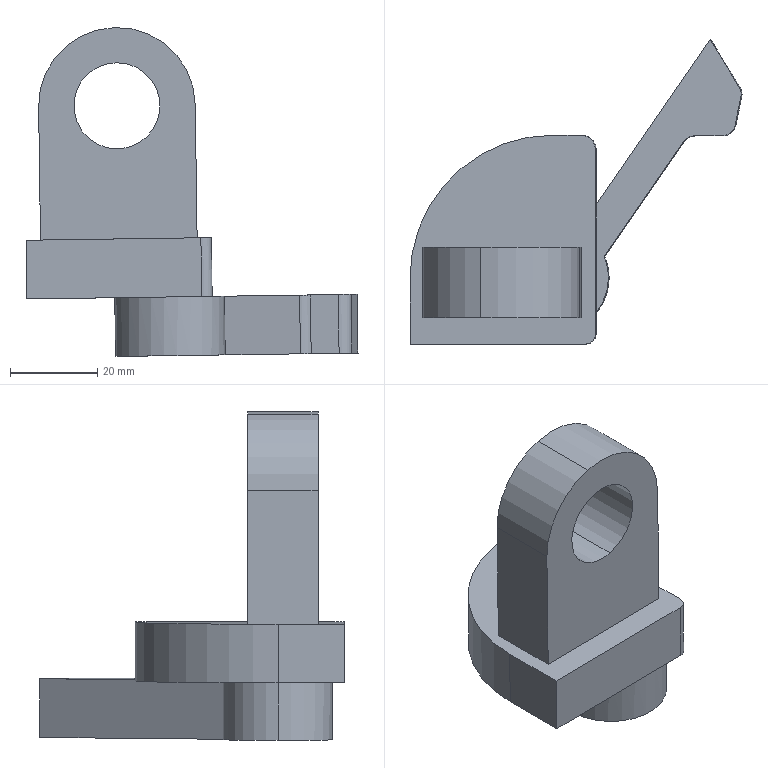Part | SolidWorks | features BaseBody 1 | 1 solid | 30 faces | box 76.312 x 69.944 x 75.61 mm | volume 59261 mm3 | plane 17 | cylinder 13 | commonest cylinder face diameters 6 x3 25.2 x3 19.8 x2 36 x2 4.8 x1 6.473 x1
STEP:
#1=CARTESIAN_POINT('',(-204.185,169.283,1047.886));
#2=VERTEX_POINT('',#1);
#3=CARTESIAN_POINT('',(-229.382,169.283,1047.53));
#4=VERTEX_POINT('',#3);
#5=CARTESIAN_POINT('',(-216.783,169.283,1047.708));
#6=DIRECTION('',(0.0141,0.,-0.9999));
#7=DIRECTION('',(0.9999,0.,0.0141));
#8=AXIS2_PLACEMENT_3D('',#5,#6,#7);
#9=CIRCLE('',#8,12.6);
#10=EDGE_CURVE('',#2,#4,#9,.T.);
#11=ORIENTED_EDGE('',*,*,#10,.F.);
#12=CARTESIAN_POINT('',(-204.375,169.283,1061.384));
#13=VERTEX_POINT('',#12);
#14=CARTESIAN_POINT('',(-204.185,169.283,1047.886));
#15=DIRECTION('',(-0.0141,0.,0.9999));
#16=VECTOR('',#15,1000.);
#17=LINE('',#14,#16);
#18=EDGE_CURVE('',#2,#13,#17,.T.);
#19=ORIENTED_EDGE('',*,*,#18,.T.);
#20=CARTESIAN_POINT('',(-207.186,161.349,1061.345));
#21=VERTEX_POINT('',#20);
#22=CARTESIAN_POINT('',(-216.974,169.283,1061.207));
#23=DIRECTION('',(0.0141,0.,-0.9999));
#24=DIRECTION('',(0.9999,0.,0.0141));
#25=AXIS2_PLACEMENT_3D('',#22,#23,#24);
#26=CIRCLE('',#25,12.6);
#27=EDGE_CURVE('',#13,#21,#26,.T.);
#28=ORIENTED_EDGE('',*,*,#27,.T.);
#29=CARTESIAN_POINT('',(-229.572,169.283,1061.029));
#30=VERTEX_POINT('',#29);
#31=CARTESIAN_POINT('',(-216.974,169.283,1061.207));
#32=DIRECTION('',(0.0141,0.,-0.9999));
#33=DIRECTION('',(0.9999,0.,0.0141));
#34=AXIS2_PLACEMENT_3D('',#31,#32,#33);
#35=CIRCLE('',#34,12.6);
#36=EDGE_CURVE('',#21,#30,#35,.T.);
#37=ORIENTED_EDGE('',*,*,#36,.T.);
#38=CARTESIAN_POINT('',(-229.382,169.283,1047.53));
#39=DIRECTION('',(-0.0141,0.,0.9999));
#40=VECTOR('',#39,1000.);
#41=LINE('',#38,#40);
#42=EDGE_CURVE('',#4,#30,#41,.T.);
#43=ORIENTED_EDGE('',*,*,#42,.F.);
#44=EDGE_LOOP('',(#11,#19,#28,#37,#43));
#45=FACE_OUTER_BOUND('',#44,.T.);
#46=CARTESIAN_POINT('',(-216.783,169.283,1047.708));
#47=DIRECTION('',(-0.0141,0.,0.9999));
#48=DIRECTION('',(-0.9999,0.,-0.0141));
#49=AXIS2_PLACEMENT_3D('',#46,#47,#48);
#50=CYLINDRICAL_SURFACE('',#49,12.6);
#51=ADVANCED_FACE('',(#45),#50,.T.);
#52=CARTESIAN_POINT('',(-210.908,180.429,1047.791));
#53=VERTEX_POINT('',#52);
#54=CARTESIAN_POINT('',(-216.783,169.283,1047.708));
#55=DIRECTION('',(0.0141,0.,-0.9999));
#56=DIRECTION('',(0.9999,0.,0.0141));
#57=AXIS2_PLACEMENT_3D('',#54,#55,#56);
#58=CIRCLE('',#57,12.6);
#59=EDGE_CURVE('',#4,#53,#58,.T.);
#60=ORIENTED_EDGE('',*,*,#59,.F.);
#61=ORIENTED_EDGE('',*,*,#42,.T.);
#62=CARTESIAN_POINT('',(-211.099,180.429,1061.289));
#63=VERTEX_POINT('',#62);
#64=CARTESIAN_POINT('',(-216.974,169.283,1061.207));
#65=DIRECTION('',(0.0141,0.,-0.9999));
#66=DIRECTION('',(0.9999,0.,0.0141));
#67=AXIS2_PLACEMENT_3D('',#64,#65,#66);
#68=CIRCLE('',#67,12.6);
#69=EDGE_CURVE('',#30,#63,#68,.T.);
#70=ORIENTED_EDGE('',*,*,#69,.T.);
#71=CARTESIAN_POINT('',(-210.908,180.429,1047.791));
#72=DIRECTION('',(-0.0141,0.,0.9999));
#73=VECTOR('',#72,1000.);
#74=LINE('',#71,#73);
#75=EDGE_CURVE('',#53,#63,#74,.T.);
#76=ORIENTED_EDGE('',*,*,#75,.F.);
#77=EDGE_LOOP('',(#60,#61,#70,#76));
#78=FACE_OUTER_BOUND('',#77,.T.);
#79=CARTESIAN_POINT('',(-216.783,169.283,1047.708));
#80=DIRECTION('',(-0.0141,0.,0.9999));
#81=DIRECTION('',(-0.9999,0.,-0.0141));
#82=AXIS2_PLACEMENT_3D('',#79,#80,#81);
#83=CYLINDRICAL_SURFACE('',#82,12.6);
#84=ADVANCED_FACE('',(#78),#83,.T.);
#85=CARTESIAN_POINT('',(-226.509,176.294,1095.578));
#86=VERTEX_POINT('',#85);
#87=CARTESIAN_POINT('',(-231.633,176.294,1114.703));
#88=VERTEX_POINT('',#87);
#89=CARTESIAN_POINT('',(-229.071,176.294,1105.14));
#90=DIRECTION('',(0.,-1.,0.));
#91=DIRECTION('',(0.9999,0.,0.0141));
#92=AXIS2_PLACEMENT_3D('',#89,#90,#91);
#93=CIRCLE('',#92,9.9);
#94=EDGE_CURVE('',#86,#88,#93,.T.);
#95=ORIENTED_EDGE('',*,*,#94,.F.);
#96=CARTESIAN_POINT('',(-226.509,160.094,1095.578));
#97=VERTEX_POINT('',#96);
#98=CARTESIAN_POINT('',(-226.509,176.294,1095.578));
#99=DIRECTION('',(0.,-1.,0.));
#100=VECTOR('',#99,1000.);
#101=LINE('',#98,#100);
#102=EDGE_CURVE('',#86,#97,#101,.T.);
#103=ORIENTED_EDGE('',*,*,#102,.T.);
#104=CARTESIAN_POINT('',(-231.633,160.094,1114.703));
#105=VERTEX_POINT('',#104);
#106=CARTESIAN_POINT('',(-229.071,160.094,1105.14));
#107=DIRECTION('',(0.,-1.,0.));
#108=DIRECTION('',(0.9999,0.,0.0141));
#109=AXIS2_PLACEMENT_3D('',#106,#107,#108);
#110=CIRCLE('',#109,9.9);
#111=EDGE_CURVE('',#97,#105,#110,.T.);
#112=ORIENTED_EDGE('',*,*,#111,.T.);
#113=CARTESIAN_POINT('',(-231.633,176.294,1114.703));
#114=DIRECTION('',(0.,-1.,0.));
#115=VECTOR('',#114,1000.);
#116=LINE('',#113,#115);
#117=EDGE_CURVE('',#88,#105,#116,.T.);
#118=ORIENTED_EDGE('',*,*,#117,.F.);
#119=EDGE_LOOP('',(#95,#103,#112,#118));
#120=FACE_OUTER_BOUND('',#119,.T.);
#121=CARTESIAN_POINT('',(-229.071,176.294,1105.14));
#122=DIRECTION('',(0.,-1.,0.));
#123=DIRECTION('',(-0.2588,0.,0.9659));
#124=AXIS2_PLACEMENT_3D('',#121,#122,#123);
#125=CYLINDRICAL_SURFACE('',#124,9.9);
#126=ADVANCED_FACE('',(#120),#125,.F.);
#127=CARTESIAN_POINT('',(-211.073,176.294,1105.394));
#128=VERTEX_POINT('',#127);
#129=CARTESIAN_POINT('',(-233.73,176.294,1122.527));
#130=VERTEX_POINT('',#129);
#131=CARTESIAN_POINT('',(-229.071,176.294,1105.14));
#132=DIRECTION('',(0.,-1.,0.));
#133=DIRECTION('',(0.9999,0.,0.0141));
#134=AXIS2_PLACEMENT_3D('',#131,#132,#133);
#135=CIRCLE('',#134,18.);
#136=EDGE_CURVE('',#128,#130,#135,.T.);
#137=ORIENTED_EDGE('',*,*,#136,.T.);
#138=CARTESIAN_POINT('',(-233.73,160.094,1122.527));
#139=VERTEX_POINT('',#138);
#140=CARTESIAN_POINT('',(-233.73,176.294,1122.527));
#141=DIRECTION('',(0.,-1.,0.));
#142=VECTOR('',#141,1000.);
#143=LINE('',#140,#142);
#144=EDGE_CURVE('',#130,#139,#143,.T.);
#145=ORIENTED_EDGE('',*,*,#144,.T.);
#146=CARTESIAN_POINT('',(-211.073,160.094,1105.394));
#147=VERTEX_POINT('',#146);
#148=CARTESIAN_POINT('',(-229.071,160.094,1105.14));
#149=DIRECTION('',(0.,-1.,0.));
#150=DIRECTION('',(0.9999,0.,0.0141));
#151=AXIS2_PLACEMENT_3D('',#148,#149,#150);
#152=CIRCLE('',#151,18.);
#153=EDGE_CURVE('',#147,#139,#152,.T.);
#154=ORIENTED_EDGE('',*,*,#153,.F.);
#155=CARTESIAN_POINT('',(-211.073,176.294,1105.394));
#156=DIRECTION('',(0.,-1.,0.));
#157=VECTOR('',#156,1000.);
#158=LINE('',#155,#157);
#159=EDGE_CURVE('',#128,#147,#158,.T.);
#160=ORIENTED_EDGE('',*,*,#159,.F.);
#161=EDGE_LOOP('',(#137,#145,#154,#160));
#162=FACE_OUTER_BOUND('',#161,.T.);
#163=CARTESIAN_POINT('',(-229.071,176.294,1105.14));
#164=DIRECTION('',(0.,-1.,0.));
#165=DIRECTION('',(-0.2588,0.,0.9659));
#166=AXIS2_PLACEMENT_3D('',#163,#164,#165);
#167=CYLINDRICAL_SURFACE('',#166,18.);
#168=ADVANCED_FACE('',(#162),#167,.T.);
#169=CARTESIAN_POINT('',(-175.066,204.386,1048.296));
#170=VERTEX_POINT('',#169);
#171=CARTESIAN_POINT('',(-178.006,201.983,1048.255));
#172=VERTEX_POINT('',#171);
#173=CARTESIAN_POINT('',(-178.006,204.983,1048.255));
#174=DIRECTION('',(0.0141,0.,-0.9999));
#175=DIRECTION('',(-0.9999,0.,-0.0141));
#176=AXIS2_PLACEMENT_3D('',#173,#174,#175);
#177=CIRCLE('',#176,3.);
#178=EDGE_CURVE('',#170,#172,#177,.T.);
#179=ORIENTED_EDGE('',*,*,#178,.F.);
#180=CARTESIAN_POINT('',(-175.257,204.386,1061.795));
#181=VERTEX_POINT('',#180);
#182=CARTESIAN_POINT('',(-175.066,204.386,1048.296));
#183=DIRECTION('',(0.0141,0.,-0.9999));
#184=VECTOR('',#183,1000.);
#185=LINE('',#182,#184);
#186=EDGE_CURVE('',#181,#170,#185,.T.);
#187=ORIENTED_EDGE('',*,*,#186,.F.);
#188=CARTESIAN_POINT('',(-178.196,201.983,1061.753));
#189=VERTEX_POINT('',#188);
#190=CARTESIAN_POINT('',(-178.196,204.983,1061.753));
#191=DIRECTION('',(-0.0141,0.,0.9999));
#192=DIRECTION('',(-0.9999,0.,-0.0141));
#193=AXIS2_PLACEMENT_3D('',#190,#191,#192);
#194=CIRCLE('',#193,3.);
#195=EDGE_CURVE('',#189,#181,#194,.T.);
#196=ORIENTED_EDGE('',*,*,#195,.F.);
#197=CARTESIAN_POINT('',(-178.006,201.983,1048.255));
#198=DIRECTION('',(-0.0141,0.,0.9999));
#199=VECTOR('',#198,1000.);
#200=LINE('',#197,#199);
#201=EDGE_CURVE('',#172,#189,#200,.T.);
#202=ORIENTED_EDGE('',*,*,#201,.F.);
#203=EDGE_LOOP('',(#179,#187,#196,#202));
#204=FACE_OUTER_BOUND('',#203,.T.);
#205=CARTESIAN_POINT('',(-178.006,204.983,1048.255));
#206=DIRECTION('',(-0.0141,0.,0.9999));
#207=DIRECTION('',(-0.9999,0.,-0.0141));
#208=AXIS2_PLACEMENT_3D('',#205,#206,#207);
#209=CYLINDRICAL_SURFACE('',#208,3.);
#210=ADVANCED_FACE('',(#204),#209,.T.);
#211=CARTESIAN_POINT('',(-184.425,201.983,1048.164));
#212=VERTEX_POINT('',#211);
#213=CARTESIAN_POINT('',(-186.893,200.688,1048.129));
#214=VERTEX_POINT('',#213);
#215=CARTESIAN_POINT('',(-184.425,198.983,1048.164));
#216=DIRECTION('',(-0.0141,0.,0.9999));
#217=DIRECTION('',(-0.9999,0.,-0.0141));
#218=AXIS2_PLACEMENT_3D('',#215,#216,#217);
#219=CIRCLE('',#218,3.);
#220=EDGE_CURVE('',#212,#214,#219,.T.);
#221=ORIENTED_EDGE('',*,*,#220,.F.);
#222=CARTESIAN_POINT('',(-184.615,201.983,1061.663));
#223=VERTEX_POINT('',#222);
#224=CARTESIAN_POINT('',(-184.425,201.983,1048.164));
#225=DIRECTION('',(0.0141,0.,-0.9999));
#226=VECTOR('',#225,1000.);
#227=LINE('',#224,#226);
#228=EDGE_CURVE('',#223,#212,#227,.T.);
#229=ORIENTED_EDGE('',*,*,#228,.F.);
#230=CARTESIAN_POINT('',(-187.083,200.688,1061.628));
#231=VERTEX_POINT('',#230);
#232=CARTESIAN_POINT('',(-184.615,198.983,1061.663));
#233=DIRECTION('',(0.0141,0.,-0.9999));
#234=DIRECTION('',(-0.9999,0.,-0.0141));
#235=AXIS2_PLACEMENT_3D('',#232,#233,#234);
#236=CIRCLE('',#235,3.);
#237=EDGE_CURVE('',#231,#223,#236,.T.);
#238=ORIENTED_EDGE('',*,*,#237,.F.);
#239=CARTESIAN_POINT('',(-187.083,200.688,1061.628));
#240=DIRECTION('',(-0.0141,0.,0.9999));
#241=VECTOR('',#240,1000.);
#242=LINE('',#239,#241);
#243=EDGE_CURVE('',#214,#231,#242,.T.);
#244=ORIENTED_EDGE('',*,*,#243,.F.);
#245=EDGE_LOOP('',(#221,#229,#238,#244));
#246=FACE_OUTER_BOUND('',#245,.T.);
#247=CARTESIAN_POINT('',(-184.425,198.983,1048.164));
#248=DIRECTION('',(0.0141,0.,-0.9999));
#249=DIRECTION('',(0.9999,0.,0.0141));
#250=AXIS2_PLACEMENT_3D('',#247,#248,#249);
#251=CYLINDRICAL_SURFACE('',#250,3.);
#252=ADVANCED_FACE('',(#246),#251,.F.);
#253=CARTESIAN_POINT('',(-174.106,213.185,1048.31));
#254=VERTEX_POINT('',#253);
#255=CARTESIAN_POINT('',(-173.72,211.014,1048.315));
#256=VERTEX_POINT('',#255);
#257=CARTESIAN_POINT('',(-176.659,211.611,1048.274));
#258=DIRECTION('',(0.0141,0.,-0.9999));
#259=DIRECTION('',(-0.9999,0.,-0.0141));
#260=AXIS2_PLACEMENT_3D('',#257,#258,#259);
#261=CIRCLE('',#260,3.);
#262=EDGE_CURVE('',#254,#256,#261,.T.);
#263=ORIENTED_EDGE('',*,*,#262,.F.);
#264=CARTESIAN_POINT('',(-174.296,213.185,1061.808));
#265=VERTEX_POINT('',#264);
#266=CARTESIAN_POINT('',(-174.106,213.185,1048.31));
#267=DIRECTION('',(0.0141,0.,-0.9999));
#268=VECTOR('',#267,1000.);
#269=LINE('',#266,#268);
#270=EDGE_CURVE('',#265,#254,#269,.T.);
#271=ORIENTED_EDGE('',*,*,#270,.F.);
#272=CARTESIAN_POINT('',(-173.91,211.014,1061.814));
#273=VERTEX_POINT('',#272);
#274=CARTESIAN_POINT('',(-176.85,211.611,1061.772));
#275=DIRECTION('',(-0.0141,0.,0.9999));
#276=DIRECTION('',(-0.9999,0.,-0.0141));
#277=AXIS2_PLACEMENT_3D('',#274,#275,#276);
#278=CIRCLE('',#277,3.);
#279=EDGE_CURVE('',#273,#265,#278,.T.);
#280=ORIENTED_EDGE('',*,*,#279,.F.);
#281=CARTESIAN_POINT('',(-173.72,211.014,1048.315));
#282=DIRECTION('',(-0.0141,0.,0.9999));
#283=VECTOR('',#282,1000.);
#284=LINE('',#281,#283);
#285=EDGE_CURVE('',#256,#273,#284,.T.);
#286=ORIENTED_EDGE('',*,*,#285,.F.);
#287=EDGE_LOOP('',(#263,#271,#280,#286));
#288=FACE_OUTER_BOUND('',#287,.T.);
#289=CARTESIAN_POINT('',(-176.659,211.611,1048.274));
#290=DIRECTION('',(-0.0141,0.,0.9999));
#291=DIRECTION('',(-0.9999,0.,-0.0141));
#292=AXIS2_PLACEMENT_3D('',#289,#290,#291);
#293=CYLINDRICAL_SURFACE('',#292,3.);
#294=ADVANCED_FACE('',(#288),#293,.T.);
#295=CARTESIAN_POINT('',(-180.792,224.039,1048.216));
#296=VERTEX_POINT('',#295);
#297=CARTESIAN_POINT('',(-178.025,219.547,1048.255));
#298=DIRECTION('',(0.5245,-0.8514,0.007398));
#299=VECTOR('',#298,1000.);
#300=LINE('',#297,#299);
#301=EDGE_CURVE('',#296,#254,#300,.T.);
#302=ORIENTED_EDGE('',*,*,#301,.T.);
#303=ORIENTED_EDGE('',*,*,#262,.T.);
#304=CARTESIAN_POINT('',(-174.428,207.529,1048.305));
#305=DIRECTION('',(-0.1991,-0.98,-0.002808));
#306=VECTOR('',#305,1000.);
#307=LINE('',#304,#306);
#308=EDGE_CURVE('',#256,#170,#307,.T.);
#309=ORIENTED_EDGE('',*,*,#308,.T.);
#310=ORIENTED_EDGE('',*,*,#178,.T.);
#311=CARTESIAN_POINT('',(-190.236,201.983,1048.082));
#312=DIRECTION('',(-0.9999,0.,-0.0141));
#313=VECTOR('',#312,1000.);
#314=LINE('',#311,#313);
#315=EDGE_CURVE('',#172,#212,#314,.T.);
#316=ORIENTED_EDGE('',*,*,#315,.T.);
#317=ORIENTED_EDGE('',*,*,#220,.T.);
#318=CARTESIAN_POINT('',(-205.184,174.201,1047.871));
#319=VERTEX_POINT('',#318);
#320=CARTESIAN_POINT('',(-194.286,189.983,1048.025));
#321=DIRECTION('',(-0.5682,-0.8228,-0.008015));
#322=VECTOR('',#321,1000.);
#323=LINE('',#320,#322);
#324=EDGE_CURVE('',#214,#319,#323,.T.);
#325=ORIENTED_EDGE('',*,*,#324,.T.);
#326=CARTESIAN_POINT('',(-216.783,169.283,1047.708));
#327=DIRECTION('',(0.0141,0.,-0.9999));
#328=DIRECTION('',(0.9999,0.,0.0141));
#329=AXIS2_PLACEMENT_3D('',#326,#327,#328);
#330=CIRCLE('',#329,12.6);
#331=EDGE_CURVE('',#319,#2,#330,.T.);
#332=ORIENTED_EDGE('',*,*,#331,.T.);
#333=ORIENTED_EDGE('',*,*,#10,.T.);
#334=ORIENTED_EDGE('',*,*,#59,.T.);
#335=CARTESIAN_POINT('',(-210.908,180.429,1047.791));
#336=DIRECTION('',(0.5682,0.8228,0.008015));
#337=VECTOR('',#336,1000.);
#338=LINE('',#335,#337);
#339=EDGE_CURVE('',#53,#296,#338,.T.);
#340=ORIENTED_EDGE('',*,*,#339,.T.);
#341=EDGE_LOOP('',(#302,#303,#309,#310,#316,#317,#325,#332,#333,#334,#340));
#342=FACE_OUTER_BOUND('',#341,.T.);
#343=CARTESIAN_POINT('',(-216.783,169.283,1047.708));
#344=DIRECTION('',(0.0141,0.,-0.9999));
#345=DIRECTION('',(0.,-1.,0.));
#346=AXIS2_PLACEMENT_3D('',#343,#344,#345);
#347=PLANE('',#346);
#348=ADVANCED_FACE('',(#342),#347,.T.);
#349=CARTESIAN_POINT('',(-174.618,207.529,1061.804));
#350=DIRECTION('',(-0.1991,-0.98,-0.002808));
#351=VECTOR('',#350,1000.);
#352=LINE('',#349,#351);
#353=EDGE_CURVE('',#273,#181,#352,.T.);
#354=ORIENTED_EDGE('',*,*,#353,.F.);
#355=ORIENTED_EDGE('',*,*,#279,.T.);
#356=CARTESIAN_POINT('',(-180.983,224.039,1061.714));
#357=VERTEX_POINT('',#356);
#358=CARTESIAN_POINT('',(-178.216,219.547,1061.753));
#359=DIRECTION('',(0.5245,-0.8514,0.007398));
#360=VECTOR('',#359,1000.);
#361=LINE('',#358,#360);
#362=EDGE_CURVE('',#357,#265,#361,.T.);
#363=ORIENTED_EDGE('',*,*,#362,.F.);
#364=CARTESIAN_POINT('',(-207.186,186.095,1061.345));
#365=VERTEX_POINT('',#364);
#366=CARTESIAN_POINT('',(-211.099,180.429,1061.289));
#367=DIRECTION('',(0.5682,0.8228,0.008015));
#368=VECTOR('',#367,1000.);
#369=LINE('',#366,#368);
#370=EDGE_CURVE('',#365,#357,#369,.T.);
#371=ORIENTED_EDGE('',*,*,#370,.F.);
#372=CARTESIAN_POINT('',(-207.186,152.929,1061.345));
#373=DIRECTION('',(0.,1.,0.));
#374=VECTOR('',#373,1000.);
#375=LINE('',#372,#374);
#376=EDGE_CURVE('',#21,#365,#375,.T.);
#377=ORIENTED_EDGE('',*,*,#376,.F.);
#378=ORIENTED_EDGE('',*,*,#27,.F.);
#379=CARTESIAN_POINT('',(-205.375,174.201,1061.37));
#380=VERTEX_POINT('',#379);
#381=CARTESIAN_POINT('',(-216.974,169.283,1061.207));
#382=DIRECTION('',(0.0141,0.,-0.9999));
#383=DIRECTION('',(0.9999,0.,0.0141));
#384=AXIS2_PLACEMENT_3D('',#381,#382,#383);
#385=CIRCLE('',#384,12.6);
#386=EDGE_CURVE('',#380,#13,#385,.T.);
#387=ORIENTED_EDGE('',*,*,#386,.F.);
#388=CARTESIAN_POINT('',(-194.476,189.983,1061.524));
#389=DIRECTION('',(-0.5682,-0.8228,-0.008015));
#390=VECTOR('',#389,1000.);
#391=LINE('',#388,#390);
#392=EDGE_CURVE('',#231,#380,#391,.T.);
#393=ORIENTED_EDGE('',*,*,#392,.F.);
#394=ORIENTED_EDGE('',*,*,#237,.T.);
#395=CARTESIAN_POINT('',(-190.426,201.983,1061.581));
#396=DIRECTION('',(-0.9999,0.,-0.0141));
#397=VECTOR('',#396,1000.);
#398=LINE('',#395,#397);
#399=EDGE_CURVE('',#189,#223,#398,.T.);
#400=ORIENTED_EDGE('',*,*,#399,.F.);
#401=ORIENTED_EDGE('',*,*,#195,.T.);
#402=EDGE_LOOP('',(#354,#355,#363,#371,#377,#378,#387,#393,#394,#400,#401));
#403=FACE_OUTER_BOUND('',#402,.T.);
#404=CARTESIAN_POINT('',(-216.974,169.283,1061.207));
#405=DIRECTION('',(0.0141,0.,-0.9999));
#406=DIRECTION('',(0.,-1.,0.));
#407=AXIS2_PLACEMENT_3D('',#404,#405,#406);
#408=PLANE('',#407);
#409=ADVANCED_FACE('',(#403),#408,.F.);
#410=ORIENTED_EDGE('',*,*,#324,.F.);
#411=ORIENTED_EDGE('',*,*,#243,.T.);
#412=ORIENTED_EDGE('',*,*,#392,.T.);
#413=CARTESIAN_POINT('',(-205.184,174.201,1047.871));
#414=DIRECTION('',(-0.0141,0.,0.9999));
#415=VECTOR('',#414,1000.);
#416=LINE('',#413,#415);
#417=EDGE_CURVE('',#319,#380,#416,.T.);
#418=ORIENTED_EDGE('',*,*,#417,.F.);
#419=EDGE_LOOP('',(#410,#411,#412,#418));
#420=FACE_OUTER_BOUND('',#419,.T.);
#421=CARTESIAN_POINT('',(-194.286,189.983,1048.025));
#422=DIRECTION('',(-0.8227,0.5683,-0.0116));
#423=DIRECTION('',(-0.0141,0.,0.9999));
#424=AXIS2_PLACEMENT_3D('',#421,#422,#423);
#425=PLANE('',#424);
#426=ADVANCED_FACE('',(#420),#425,.F.);
#427=ORIENTED_EDGE('',*,*,#399,.T.);
#428=ORIENTED_EDGE('',*,*,#228,.T.);
#429=ORIENTED_EDGE('',*,*,#315,.F.);
#430=ORIENTED_EDGE('',*,*,#201,.T.);
#431=EDGE_LOOP('',(#427,#428,#429,#430));
#432=FACE_OUTER_BOUND('',#431,.T.);
#433=CARTESIAN_POINT('',(-190.236,201.983,1048.082));
#434=DIRECTION('',(0.,1.,0.));
#435=DIRECTION('',(1.,0.,0.));
#436=AXIS2_PLACEMENT_3D('',#433,#434,#435);
#437=PLANE('',#436);
#438=ADVANCED_FACE('',(#432),#437,.F.);
#439=ORIENTED_EDGE('',*,*,#308,.F.);
#440=ORIENTED_EDGE('',*,*,#285,.T.);
#441=ORIENTED_EDGE('',*,*,#353,.T.);
#442=ORIENTED_EDGE('',*,*,#186,.T.);
#443=EDGE_LOOP('',(#439,#440,#441,#442));
#444=FACE_OUTER_BOUND('',#443,.T.);
#445=CARTESIAN_POINT('',(-174.428,207.529,1048.305));
#446=DIRECTION('',(-0.9799,0.1991,-0.01382));
#447=DIRECTION('',(-0.0141,0.,0.9999));
#448=AXIS2_PLACEMENT_3D('',#445,#446,#447);
#449=PLANE('',#448);
#450=ADVANCED_FACE('',(#444),#449,.F.);
#451=ORIENTED_EDGE('',*,*,#362,.T.);
#452=ORIENTED_EDGE('',*,*,#270,.T.);
#453=ORIENTED_EDGE('',*,*,#301,.F.);
#454=CARTESIAN_POINT('',(-180.792,224.039,1048.216));
#455=DIRECTION('',(-0.0141,0.,0.9999));
#456=VECTOR('',#455,1000.);
#457=LINE('',#454,#456);
#458=EDGE_CURVE('',#296,#357,#457,.T.);
#459=ORIENTED_EDGE('',*,*,#458,.T.);
#460=EDGE_LOOP('',(#451,#452,#453,#459));
#461=FACE_OUTER_BOUND('',#460,.T.);
#462=CARTESIAN_POINT('',(-178.025,219.547,1048.255));
#463=DIRECTION('',(-0.8513,-0.5246,-0.01201));
#464=DIRECTION('',(-0.5246,0.8513,0.));
#465=AXIS2_PLACEMENT_3D('',#462,#463,#464);
#466=PLANE('',#465);
#467=ADVANCED_FACE('',(#461),#466,.F.);
#468=CARTESIAN_POINT('',(-211.099,180.429,1061.289));
#469=DIRECTION('',(0.5682,0.8228,0.008015));
#470=VECTOR('',#469,1000.);
#471=LINE('',#468,#470);
#472=EDGE_CURVE('',#63,#365,#471,.T.);
#473=ORIENTED_EDGE('',*,*,#472,.T.);
#474=ORIENTED_EDGE('',*,*,#370,.T.);
#475=ORIENTED_EDGE('',*,*,#458,.F.);
#476=ORIENTED_EDGE('',*,*,#339,.F.);
#477=ORIENTED_EDGE('',*,*,#75,.T.);
#478=EDGE_LOOP('',(#473,#474,#475,#476,#477));
#479=FACE_OUTER_BOUND('',#478,.T.);
#480=CARTESIAN_POINT('',(-210.908,180.429,1047.791));
#481=DIRECTION('',(0.8227,-0.5683,0.0116));
#482=DIRECTION('',(0.,-0.02042,-0.9998));
#483=AXIS2_PLACEMENT_3D('',#480,#481,#482);
#484=PLANE('',#483);
#485=ADVANCED_FACE('',(#479),#484,.F.);
#486=CARTESIAN_POINT('',(-207.186,156.494,1061.345));
#487=VERTEX_POINT('',#486);
#488=CARTESIAN_POINT('',(-209.586,154.094,1061.311));
#489=VERTEX_POINT('',#488);
#490=CARTESIAN_POINT('',(-209.586,156.494,1061.311));
#491=DIRECTION('',(0.0141,0.,-0.9999));
#492=DIRECTION('',(0.9999,0.,0.0141));
#493=AXIS2_PLACEMENT_3D('',#490,#491,#492);
#494=CIRCLE('',#493,2.4);
#495=EDGE_CURVE('',#487,#489,#494,.T.);
#496=ORIENTED_EDGE('',*,*,#495,.F.);
#497=CARTESIAN_POINT('',(-207.376,156.494,1074.843));
#498=VERTEX_POINT('',#497);
#499=CARTESIAN_POINT('',(-207.186,156.494,1061.345));
#500=DIRECTION('',(0.0141,0.,-0.9999));
#501=VECTOR('',#500,1000.);
#502=LINE('',#499,#501);
#503=EDGE_CURVE('',#498,#487,#502,.T.);
#504=ORIENTED_EDGE('',*,*,#503,.F.);
#505=CARTESIAN_POINT('',(-209.776,154.094,1074.809));
#506=VERTEX_POINT('',#505);
#507=CARTESIAN_POINT('',(-209.776,156.494,1074.809));
#508=DIRECTION('',(-0.0141,0.,0.9999));
#509=DIRECTION('',(0.9999,0.,0.0141));
#510=AXIS2_PLACEMENT_3D('',#507,#508,#509);
#511=CIRCLE('',#510,2.4);
#512=EDGE_CURVE('',#506,#498,#511,.T.);
#513=ORIENTED_EDGE('',*,*,#512,.F.);
#514=CARTESIAN_POINT('',(-209.586,154.094,1061.311));
#515=DIRECTION('',(-0.0141,0.,0.9999));
#516=VECTOR('',#515,1000.);
#517=LINE('',#514,#516);
#518=EDGE_CURVE('',#489,#506,#517,.T.);
#519=ORIENTED_EDGE('',*,*,#518,.F.);
#520=EDGE_LOOP('',(#496,#504,#513,#519));
#521=FACE_OUTER_BOUND('',#520,.T.);
#522=CARTESIAN_POINT('',(-209.586,156.494,1061.311));
#523=DIRECTION('',(-0.0141,0.,0.9999));
#524=DIRECTION('',(-0.9999,0.,-0.0141));
#525=AXIS2_PLACEMENT_3D('',#522,#523,#524);
#526=CYLINDRICAL_SURFACE('',#525,2.4);
#527=ADVANCED_FACE('',(#521),#526,.T.);
#528=CARTESIAN_POINT('',(-229.071,160.094,1105.14));
#529=DIRECTION('',(0.,-1.,0.));
#530=DIRECTION('',(0.9999,0.,0.0141));
#531=AXIS2_PLACEMENT_3D('',#528,#529,#530);
#532=CIRCLE('',#531,9.9);
#533=EDGE_CURVE('',#105,#97,#532,.T.);
#534=ORIENTED_EDGE('',*,*,#533,.F.);
#535=ORIENTED_EDGE('',*,*,#111,.F.);
#536=EDGE_LOOP('',(#534,#535));
#537=FACE_BOUND('',#536,.T.);
#538=CARTESIAN_POINT('',(-247.069,160.094,1104.886));
#539=VERTEX_POINT('',#538);
#540=CARTESIAN_POINT('',(-246.638,160.094,1074.289));
#541=VERTEX_POINT('',#540);
#542=CARTESIAN_POINT('',(-247.069,160.094,1104.886));
#543=DIRECTION('',(0.0141,0.,-0.9999));
#544=VECTOR('',#543,1000.);
#545=LINE('',#542,#544);
#546=EDGE_CURVE('',#539,#541,#545,.T.);
#547=ORIENTED_EDGE('',*,*,#546,.T.);
#548=CARTESIAN_POINT('',(-210.641,160.094,1074.797));
#549=VERTEX_POINT('',#548);
#550=CARTESIAN_POINT('',(-251.137,160.094,1074.226));
#551=DIRECTION('',(0.9999,0.,0.0141));
#552=VECTOR('',#551,1000.);
#553=LINE('',#550,#552);
#554=EDGE_CURVE('',#541,#549,#553,.T.);
#555=ORIENTED_EDGE('',*,*,#554,.T.);
#556=CARTESIAN_POINT('',(-210.573,160.094,1069.937));
#557=DIRECTION('',(-0.0141,0.,0.9999));
#558=VECTOR('',#557,1000.);
#559=LINE('',#556,#558);
#560=EDGE_CURVE('',#549,#147,#559,.T.);
#561=ORIENTED_EDGE('',*,*,#560,.T.);
#562=ORIENTED_EDGE('',*,*,#153,.T.);
#563=CARTESIAN_POINT('',(-229.071,160.094,1105.14));
#564=DIRECTION('',(0.,-1.,0.));
#565=DIRECTION('',(0.9999,0.,0.0141));
#566=AXIS2_PLACEMENT_3D('',#563,#564,#565);
#567=CIRCLE('',#566,18.);
#568=EDGE_CURVE('',#139,#539,#567,.T.);
#569=ORIENTED_EDGE('',*,*,#568,.T.);
#570=EDGE_LOOP('',(#547,#555,#561,#562,#569));
#571=FACE_OUTER_BOUND('',#570,.T.);
#572=CARTESIAN_POINT('',(-229.071,160.094,1105.14));
#573=DIRECTION('',(0.,-1.,0.));
#574=DIRECTION('',(0.,0.,-1.));
#575=AXIS2_PLACEMENT_3D('',#572,#573,#574);
#576=PLANE('',#575);
#577=ADVANCED_FACE('',(#537,#571),#576,.T.);
#578=CARTESIAN_POINT('',(-229.071,176.294,1105.14));
#579=DIRECTION('',(0.,-1.,0.));
#580=DIRECTION('',(0.9999,0.,0.0141));
#581=AXIS2_PLACEMENT_3D('',#578,#579,#580);
#582=CIRCLE('',#581,9.9);
#583=EDGE_CURVE('',#88,#86,#582,.T.);
#584=ORIENTED_EDGE('',*,*,#583,.T.);
#585=ORIENTED_EDGE('',*,*,#94,.T.);
#586=EDGE_LOOP('',(#584,#585));
#587=FACE_BOUND('',#586,.T.);
#588=CARTESIAN_POINT('',(-246.638,176.294,1074.289));
#589=VERTEX_POINT('',#588);
#590=CARTESIAN_POINT('',(-210.641,176.294,1074.797));
#591=VERTEX_POINT('',#590);
#592=CARTESIAN_POINT('',(-251.137,176.294,1074.226));
#593=DIRECTION('',(0.9999,0.,0.0141));
#594=VECTOR('',#593,1000.);
#595=LINE('',#592,#594);
#596=EDGE_CURVE('',#589,#591,#595,.T.);
#597=ORIENTED_EDGE('',*,*,#596,.F.);
#598=CARTESIAN_POINT('',(-247.069,176.294,1104.886));
#599=VERTEX_POINT('',#598);
#600=CARTESIAN_POINT('',(-247.069,176.294,1104.886));
#601=DIRECTION('',(0.0141,0.,-0.9999));
#602=VECTOR('',#601,1000.);
#603=LINE('',#600,#602);
#604=EDGE_CURVE('',#599,#589,#603,.T.);
#605=ORIENTED_EDGE('',*,*,#604,.F.);
#606=CARTESIAN_POINT('',(-229.071,176.294,1105.14));
#607=DIRECTION('',(0.,-1.,0.));
#608=DIRECTION('',(0.9999,0.,0.0141));
#609=AXIS2_PLACEMENT_3D('',#606,#607,#608);
#610=CIRCLE('',#609,18.);
#611=EDGE_CURVE('',#130,#599,#610,.T.);
#612=ORIENTED_EDGE('',*,*,#611,.F.);
#613=ORIENTED_EDGE('',*,*,#136,.F.);
#614=CARTESIAN_POINT('',(-210.573,176.294,1069.937));
#615=DIRECTION('',(-0.0141,0.,0.9999));
#616=VECTOR('',#615,1000.);
#617=LINE('',#614,#616);
#618=EDGE_CURVE('',#591,#128,#617,.T.);
#619=ORIENTED_EDGE('',*,*,#618,.F.);
#620=EDGE_LOOP('',(#597,#605,#612,#613,#619));
#621=FACE_OUTER_BOUND('',#620,.T.);
#622=CARTESIAN_POINT('',(-229.071,176.294,1105.14));
#623=DIRECTION('',(0.,-1.,0.));
#624=DIRECTION('',(0.,0.,-1.));
#625=AXIS2_PLACEMENT_3D('',#622,#623,#624);
#626=PLANE('',#625);
#627=ADVANCED_FACE('',(#587,#621),#626,.F.);
#628=ORIENTED_EDGE('',*,*,#560,.F.);
#629=CARTESIAN_POINT('',(-210.641,152.929,1074.797));
#630=DIRECTION('',(0.,1.,0.));
#631=VECTOR('',#630,1000.);
#632=LINE('',#629,#631);
#633=EDGE_CURVE('',#549,#591,#632,.T.);
#634=ORIENTED_EDGE('',*,*,#633,.T.);
#635=ORIENTED_EDGE('',*,*,#618,.T.);
#636=ORIENTED_EDGE('',*,*,#159,.T.);
#637=EDGE_LOOP('',(#628,#634,#635,#636));
#638=FACE_OUTER_BOUND('',#637,.T.);
#639=CARTESIAN_POINT('',(-210.573,176.294,1069.937));
#640=DIRECTION('',(0.9999,0.,0.0141));
#641=DIRECTION('',(0.,-1.,0.));
#642=AXIS2_PLACEMENT_3D('',#639,#640,#641);
#643=PLANE('',#642);
#644=ADVANCED_FACE('',(#638),#643,.T.);
#645=ORIENTED_EDGE('',*,*,#604,.T.);
#646=CARTESIAN_POINT('',(-246.638,152.929,1074.289));
#647=DIRECTION('',(0.,-1.,0.));
#648=VECTOR('',#647,1000.);
#649=LINE('',#646,#648);
#650=EDGE_CURVE('',#589,#541,#649,.T.);
#651=ORIENTED_EDGE('',*,*,#650,.T.);
#652=ORIENTED_EDGE('',*,*,#546,.F.);
#653=CARTESIAN_POINT('',(-247.069,176.294,1104.886));
#654=DIRECTION('',(0.,-1.,0.));
#655=VECTOR('',#654,1000.);
#656=LINE('',#653,#655);
#657=EDGE_CURVE('',#599,#539,#656,.T.);
#658=ORIENTED_EDGE('',*,*,#657,.F.);
#659=EDGE_LOOP('',(#645,#651,#652,#658));
#660=FACE_OUTER_BOUND('',#659,.T.);
#661=CARTESIAN_POINT('',(-247.069,176.294,1104.886));
#662=DIRECTION('',(-0.9999,0.,-0.0141));
#663=DIRECTION('',(-0.0141,0.,0.9999));
#664=AXIS2_PLACEMENT_3D('',#661,#662,#663);
#665=PLANE('',#664);
#666=ADVANCED_FACE('',(#660),#665,.T.);
#667=ORIENTED_EDGE('',*,*,#36,.F.);
#668=CARTESIAN_POINT('',(-207.186,152.929,1061.345));
#669=DIRECTION('',(0.,1.,0.));
#670=VECTOR('',#669,1000.);
#671=LINE('',#668,#670);
#672=EDGE_CURVE('',#487,#21,#671,.T.);
#673=ORIENTED_EDGE('',*,*,#672,.F.);
#674=ORIENTED_EDGE('',*,*,#495,.T.);
#675=CARTESIAN_POINT('',(-249.782,154.094,1060.744));
#676=VERTEX_POINT('',#675);
#677=CARTESIAN_POINT('',(-250.947,154.094,1060.727));
#678=DIRECTION('',(0.9999,0.,0.0141));
#679=VECTOR('',#678,1000.);
#680=LINE('',#677,#679);
#681=EDGE_CURVE('',#676,#489,#680,.T.);
#682=ORIENTED_EDGE('',*,*,#681,.F.);
#683=CARTESIAN_POINT('',(-249.782,169.283,1060.744));
#684=VERTEX_POINT('',#683);
#685=CARTESIAN_POINT('',(-249.782,152.929,1060.744));
#686=DIRECTION('',(0.,-1.,0.));
#687=VECTOR('',#686,1000.);
#688=LINE('',#685,#687);
#689=EDGE_CURVE('',#684,#676,#688,.T.);
#690=ORIENTED_EDGE('',*,*,#689,.F.);
#691=CARTESIAN_POINT('',(-216.974,202.094,1061.207));
#692=VERTEX_POINT('',#691);
#693=CARTESIAN_POINT('',(-216.974,169.283,1061.207));
#694=DIRECTION('',(-0.0141,0.,0.9999));
#695=DIRECTION('',(0.9999,0.,0.0141));
#696=AXIS2_PLACEMENT_3D('',#693,#694,#695);
#697=CIRCLE('',#696,32.811);
#698=EDGE_CURVE('',#692,#684,#697,.T.);
#699=ORIENTED_EDGE('',*,*,#698,.F.);
#700=CARTESIAN_POINT('',(-210.422,202.094,1061.299));
#701=VERTEX_POINT('',#700);
#702=CARTESIAN_POINT('',(-250.947,202.094,1060.727));
#703=DIRECTION('',(-0.9999,0.,-0.0141));
#704=VECTOR('',#703,1000.);
#705=LINE('',#702,#704);
#706=EDGE_CURVE('',#701,#692,#705,.T.);
#707=ORIENTED_EDGE('',*,*,#706,.F.);
#708=CARTESIAN_POINT('',(-207.186,198.858,1061.345));
#709=VERTEX_POINT('',#708);
#710=CARTESIAN_POINT('',(-210.422,198.858,1061.299));
#711=DIRECTION('',(-0.0141,0.,0.9999));
#712=DIRECTION('',(0.9999,0.,0.0141));
#713=AXIS2_PLACEMENT_3D('',#710,#711,#712);
#714=CIRCLE('',#713,3.236);
#715=EDGE_CURVE('',#709,#701,#714,.T.);
#716=ORIENTED_EDGE('',*,*,#715,.F.);
#717=CARTESIAN_POINT('',(-207.186,152.929,1061.345));
#718=DIRECTION('',(0.,1.,0.));
#719=VECTOR('',#718,1000.);
#720=LINE('',#717,#719);
#721=EDGE_CURVE('',#365,#709,#720,.T.);
#722=ORIENTED_EDGE('',*,*,#721,.F.);
#723=ORIENTED_EDGE('',*,*,#472,.F.);
#724=ORIENTED_EDGE('',*,*,#69,.F.);
#725=EDGE_LOOP('',(#667,#673,#674,#682,#690,#699,#707,#716,#722,#723,#724));
#726=FACE_OUTER_BOUND('',#725,.T.);
#727=CARTESIAN_POINT('',(-250.947,152.929,1060.727));
#728=DIRECTION('',(-0.0141,0.,0.9999));
#729=DIRECTION('',(0.,1.,0.));
#730=AXIS2_PLACEMENT_3D('',#727,#728,#729);
#731=PLANE('',#730);
#732=ADVANCED_FACE('',(#726),#731,.F.);
#733=CARTESIAN_POINT('',(-217.164,202.094,1074.705));
#734=VERTEX_POINT('',#733);
#735=CARTESIAN_POINT('',(-249.972,169.283,1074.242));
#736=VERTEX_POINT('',#735);
#737=CARTESIAN_POINT('',(-217.164,169.283,1074.705));
#738=DIRECTION('',(-0.0141,0.,0.9999));
#739=DIRECTION('',(0.9999,0.,0.0141));
#740=AXIS2_PLACEMENT_3D('',#737,#738,#739);
#741=CIRCLE('',#740,32.811);
#742=EDGE_CURVE('',#734,#736,#741,.T.);
#743=ORIENTED_EDGE('',*,*,#742,.F.);
#744=CARTESIAN_POINT('',(-216.974,202.094,1061.207));
#745=DIRECTION('',(-0.0141,0.,0.9999));
#746=VECTOR('',#745,1000.);
#747=LINE('',#744,#746);
#748=EDGE_CURVE('',#692,#734,#747,.T.);
#749=ORIENTED_EDGE('',*,*,#748,.F.);
#750=ORIENTED_EDGE('',*,*,#698,.T.);
#751=CARTESIAN_POINT('',(-249.782,169.283,1060.744));
#752=DIRECTION('',(-0.0141,0.,0.9999));
#753=VECTOR('',#752,1000.);
#754=LINE('',#751,#753);
#755=EDGE_CURVE('',#684,#736,#754,.T.);
#756=ORIENTED_EDGE('',*,*,#755,.T.);
#757=EDGE_LOOP('',(#743,#749,#750,#756));
#758=FACE_OUTER_BOUND('',#757,.T.);
#759=CARTESIAN_POINT('',(-216.974,169.283,1061.207));
#760=DIRECTION('',(-0.0141,0.,0.9999));
#761=DIRECTION('',(-0.9999,0.,-0.0141));
#762=AXIS2_PLACEMENT_3D('',#759,#760,#761);
#763=CYLINDRICAL_SURFACE('',#762,32.811);
#764=ADVANCED_FACE('',(#758),#763,.T.);
#765=CARTESIAN_POINT('',(-210.612,202.094,1074.798));
#766=VERTEX_POINT('',#765);
#767=CARTESIAN_POINT('',(-251.137,202.094,1074.226));
#768=DIRECTION('',(-0.9999,0.,-0.0141));
#769=VECTOR('',#768,1000.);
#770=LINE('',#767,#769);
#771=EDGE_CURVE('',#766,#734,#770,.T.);
#772=ORIENTED_EDGE('',*,*,#771,.F.);
#773=CARTESIAN_POINT('',(-210.422,202.094,1061.299));
#774=DIRECTION('',(-0.0141,0.,0.9999));
#775=VECTOR('',#774,1000.);
#776=LINE('',#773,#775);
#777=EDGE_CURVE('',#701,#766,#776,.T.);
#778=ORIENTED_EDGE('',*,*,#777,.F.);
#779=ORIENTED_EDGE('',*,*,#706,.T.);
#780=ORIENTED_EDGE('',*,*,#748,.T.);
#781=EDGE_LOOP('',(#772,#778,#779,#780));
#782=FACE_OUTER_BOUND('',#781,.T.);
#783=CARTESIAN_POINT('',(-210.422,202.094,1061.299));
#784=DIRECTION('',(0.,1.,0.));
#785=DIRECTION('',(1.,0.,0.));
#786=AXIS2_PLACEMENT_3D('',#783,#784,#785);
#787=PLANE('',#786);
#788=ADVANCED_FACE('',(#782),#787,.T.);
#789=CARTESIAN_POINT('',(-207.376,198.858,1074.843));
#790=VERTEX_POINT('',#789);
#791=CARTESIAN_POINT('',(-210.612,198.858,1074.798));
#792=DIRECTION('',(-0.0141,0.,0.9999));
#793=DIRECTION('',(0.9999,0.,0.0141));
#794=AXIS2_PLACEMENT_3D('',#791,#792,#793);
#795=CIRCLE('',#794,3.236);
#796=EDGE_CURVE('',#790,#766,#795,.T.);
#797=ORIENTED_EDGE('',*,*,#796,.F.);
#798=CARTESIAN_POINT('',(-207.186,198.858,1061.345));
#799=DIRECTION('',(-0.0141,0.,0.9999));
#800=VECTOR('',#799,1000.);
#801=LINE('',#798,#800);
#802=EDGE_CURVE('',#709,#790,#801,.T.);
#803=ORIENTED_EDGE('',*,*,#802,.F.);
#804=ORIENTED_EDGE('',*,*,#715,.T.);
#805=ORIENTED_EDGE('',*,*,#777,.T.);
#806=EDGE_LOOP('',(#797,#803,#804,#805));
#807=FACE_OUTER_BOUND('',#806,.T.);
#808=CARTESIAN_POINT('',(-210.422,198.858,1061.299));
#809=DIRECTION('',(-0.0141,0.,0.9999));
#810=DIRECTION('',(-0.9999,0.,-0.0141));
#811=AXIS2_PLACEMENT_3D('',#808,#809,#810);
#812=CYLINDRICAL_SURFACE('',#811,3.236);
#813=ADVANCED_FACE('',(#807),#812,.T.);
#814=CARTESIAN_POINT('',(-207.376,152.929,1074.843));
#815=DIRECTION('',(0.,1.,0.));
#816=VECTOR('',#815,1000.);
#817=LINE('',#814,#816);
#818=EDGE_CURVE('',#498,#790,#817,.T.);
#819=ORIENTED_EDGE('',*,*,#818,.F.);
#820=ORIENTED_EDGE('',*,*,#503,.T.);
#821=ORIENTED_EDGE('',*,*,#672,.T.);
#822=ORIENTED_EDGE('',*,*,#376,.T.);
#823=ORIENTED_EDGE('',*,*,#721,.T.);
#824=ORIENTED_EDGE('',*,*,#802,.T.);
#825=EDGE_LOOP('',(#819,#820,#821,#822,#823,#824));
#826=FACE_OUTER_BOUND('',#825,.T.);
#827=CARTESIAN_POINT('',(-207.186,146.594,1061.345));
#828=DIRECTION('',(0.9999,0.,0.0141));
#829=DIRECTION('',(0.,-1.,0.));
#830=AXIS2_PLACEMENT_3D('',#827,#828,#829);
#831=PLANE('',#830);
#832=ADVANCED_FACE('',(#826),#831,.T.);
#833=ORIENTED_EDGE('',*,*,#681,.T.);
#834=ORIENTED_EDGE('',*,*,#518,.T.);
#835=CARTESIAN_POINT('',(-249.972,154.094,1074.242));
#836=VERTEX_POINT('',#835);
#837=CARTESIAN_POINT('',(-251.137,154.094,1074.226));
#838=DIRECTION('',(0.9999,0.,0.0141));
#839=VECTOR('',#838,1000.);
#840=LINE('',#837,#839);
#841=EDGE_CURVE('',#836,#506,#840,.T.);
#842=ORIENTED_EDGE('',*,*,#841,.F.);
#843=CARTESIAN_POINT('',(-249.782,154.094,1060.744));
#844=DIRECTION('',(-0.0141,0.,0.9999));
#845=VECTOR('',#844,1000.);
#846=LINE('',#843,#845);
#847=EDGE_CURVE('',#676,#836,#846,.T.);
#848=ORIENTED_EDGE('',*,*,#847,.F.);
#849=EDGE_LOOP('',(#833,#834,#842,#848));
#850=FACE_OUTER_BOUND('',#849,.T.);
#851=CARTESIAN_POINT('',(-250.947,154.094,1060.727));
#852=DIRECTION('',(0.,-1.,0.));
#853=DIRECTION('',(0.,0.,-1.));
#854=AXIS2_PLACEMENT_3D('',#851,#852,#853);
#855=PLANE('',#854);
#856=ADVANCED_FACE('',(#850),#855,.T.);
#857=CARTESIAN_POINT('',(-249.972,152.929,1074.242));
#858=DIRECTION('',(0.,-1.,0.));
#859=VECTOR('',#858,1000.);
#860=LINE('',#857,#859);
#861=EDGE_CURVE('',#736,#836,#860,.T.);
#862=ORIENTED_EDGE('',*,*,#861,.F.);
#863=ORIENTED_EDGE('',*,*,#755,.F.);
#864=ORIENTED_EDGE('',*,*,#689,.T.);
#865=ORIENTED_EDGE('',*,*,#847,.T.);
#866=EDGE_LOOP('',(#862,#863,#864,#865));
#867=FACE_OUTER_BOUND('',#866,.T.);
#868=CARTESIAN_POINT('',(-249.782,169.283,1060.744));
#869=DIRECTION('',(-0.9999,0.,-0.0141));
#870=DIRECTION('',(-0.0141,0.,0.9999));
#871=AXIS2_PLACEMENT_3D('',#868,#869,#870);
#872=PLANE('',#871);
#873=ADVANCED_FACE('',(#867),#872,.T.);
#874=ORIENTED_EDGE('',*,*,#650,.F.);
#875=ORIENTED_EDGE('',*,*,#596,.T.);
#876=ORIENTED_EDGE('',*,*,#633,.F.);
#877=ORIENTED_EDGE('',*,*,#554,.F.);
#878=EDGE_LOOP('',(#874,#875,#876,#877));
#879=FACE_BOUND('',#878,.T.);
#880=ORIENTED_EDGE('',*,*,#841,.T.);
#881=ORIENTED_EDGE('',*,*,#512,.T.);
#882=ORIENTED_EDGE('',*,*,#818,.T.);
#883=ORIENTED_EDGE('',*,*,#796,.T.);
#884=ORIENTED_EDGE('',*,*,#771,.T.);
#885=ORIENTED_EDGE('',*,*,#742,.T.);
#886=ORIENTED_EDGE('',*,*,#861,.T.);
#887=EDGE_LOOP('',(#880,#881,#882,#883,#884,#885,#886));
#888=FACE_OUTER_BOUND('',#887,.T.);
#889=CARTESIAN_POINT('',(-251.137,152.929,1074.226));
#890=DIRECTION('',(-0.0141,0.,0.9999));
#891=DIRECTION('',(0.,1.,0.));
#892=AXIS2_PLACEMENT_3D('',#889,#890,#891);
#893=PLANE('',#892);
#894=ADVANCED_FACE('',(#879,#888),#893,.T.);
#895=ORIENTED_EDGE('',*,*,#144,.F.);
#896=ORIENTED_EDGE('',*,*,#611,.T.);
#897=ORIENTED_EDGE('',*,*,#657,.T.);
#898=ORIENTED_EDGE('',*,*,#568,.F.);
#899=EDGE_LOOP('',(#895,#896,#897,#898));
#900=FACE_OUTER_BOUND('',#899,.T.);
#901=CARTESIAN_POINT('',(-229.071,176.294,1105.14));
#902=DIRECTION('',(0.,-1.,0.));
#903=DIRECTION('',(-0.2588,0.,0.9659));
#904=AXIS2_PLACEMENT_3D('',#901,#902,#903);
#905=CYLINDRICAL_SURFACE('',#904,18.);
#906=ADVANCED_FACE('',(#900),#905,.T.);
#907=ORIENTED_EDGE('',*,*,#102,.F.);
#908=ORIENTED_EDGE('',*,*,#583,.F.);
#909=ORIENTED_EDGE('',*,*,#117,.T.);
#910=ORIENTED_EDGE('',*,*,#533,.T.);
#911=EDGE_LOOP('',(#907,#908,#909,#910));
#912=FACE_OUTER_BOUND('',#911,.T.);
#913=CARTESIAN_POINT('',(-229.071,176.294,1105.14));
#914=DIRECTION('',(0.,-1.,0.));
#915=DIRECTION('',(-0.2588,0.,0.9659));
#916=AXIS2_PLACEMENT_3D('',#913,#914,#915);
#917=CYLINDRICAL_SURFACE('',#916,9.9);
#918=ADVANCED_FACE('',(#912),#917,.F.);
#919=ORIENTED_EDGE('',*,*,#18,.F.);
#920=ORIENTED_EDGE('',*,*,#331,.F.);
#921=ORIENTED_EDGE('',*,*,#417,.T.);
#922=ORIENTED_EDGE('',*,*,#386,.T.);
#923=EDGE_LOOP('',(#919,#920,#921,#922));
#924=FACE_OUTER_BOUND('',#923,.T.);
#925=CARTESIAN_POINT('',(-216.783,169.283,1047.708));
#926=DIRECTION('',(-0.0141,0.,0.9999));
#927=DIRECTION('',(-0.9999,0.,-0.0141));
#928=AXIS2_PLACEMENT_3D('',#925,#926,#927);
#929=CYLINDRICAL_SURFACE('',#928,12.6);
#930=ADVANCED_FACE('',(#924),#929,.T.);
#931=CLOSED_SHELL('',(#51,#84,#126,#168,#210,#252,#294,#348,#409,#426,#438,#450,#467,#485,#527,#577,#627,#644,#666,#732,#764,#788,#813,#832,#856,#873,#894,#906,#918,#930));
#932=MANIFOLD_SOLID_BREP('',#931);
#933=CARTESIAN_POINT('',(0.,0.,0.));
#934=DIRECTION('',(0.,0.,1.));
#935=DIRECTION('',(1.,0.,0.));
#936=AXIS2_PLACEMENT_3D('',#933,#934,#935);
#937=(LENGTH_UNIT()NAMED_UNIT(*)SI_UNIT(.MILLI.,.METRE.));
#938=UNCERTAINTY_MEASURE_WITH_UNIT(LENGTH_MEASURE(0.00001),#937,'','');
#939=(NAMED_UNIT(*)PLANE_ANGLE_UNIT()SI_UNIT($,.RADIAN.));
#940=(NAMED_UNIT(*)SI_UNIT($,.STERADIAN.)SOLID_ANGLE_UNIT());
#941=(GEOMETRIC_REPRESENTATION_CONTEXT(3)GLOBAL_UNCERTAINTY_ASSIGNED_CONTEXT((#938))GLOBAL_UNIT_ASSIGNED_CONTEXT((#937,#939,#940))REPRESENTATION_CONTEXT('',''));
#942=ADVANCED_BREP_SHAPE_REPRESENTATION('',(#932,#936),#941);